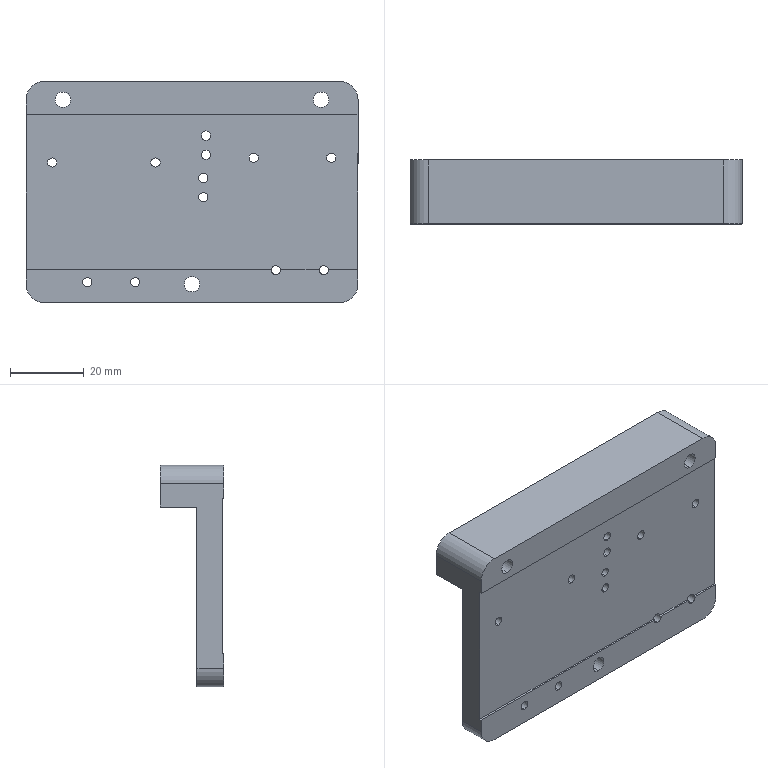Part | SolidWorks | features ICE 4, HoleWzd 2, Extrusion 1, Fillet 1 | 1 solid | 57 faces | box 90 x 17.28 x 60 mm | volume 45456 mm3 | cylinder 40 | plane 17 | commonest cylinder face diameters 2.5 x24 4.2 x6 7.5 x6 10 x4